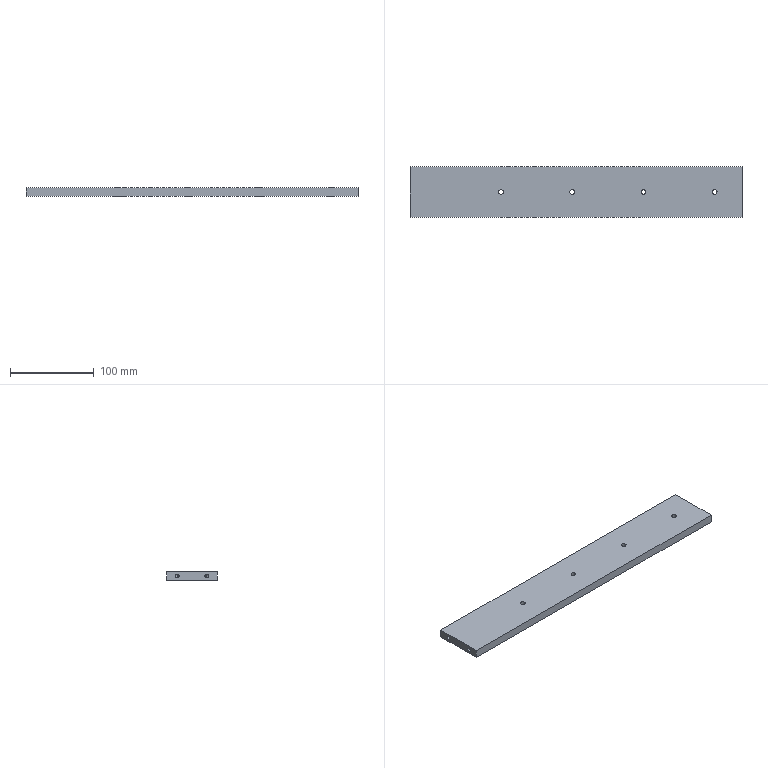Part | SolidWorks | features HoleWzd 2, Extrusion 1, MirrorPattern 1 | 1 solid | 42 faces | box 396 x 60 x 10 mm | volume 234690 mm3 | cylinder 24 | plane 10 | cone 8 | commonest cylinder face diameters 4.2 x8 5.5 x8 10 x8
STEP:
#1=CARTESIAN_POINT('',(185.6,17.5,7.1));
#2=VERTEX_POINT('',#1);
#3=CARTESIAN_POINT('',(185.6,17.5,2.9));
#4=VERTEX_POINT('',#3);
#5=CARTESIAN_POINT('',(185.6,17.5,5.));
#6=DIRECTION('',(1.,0.,0.));
#7=DIRECTION('',(0.,0.,-1.));
#8=AXIS2_PLACEMENT_3D('',#5,#6,#7);
#9=CIRCLE('',#8,2.1);
#10=EDGE_CURVE('',#2,#4,#9,.T.);
#11=ORIENTED_EDGE('',*,*,#10,.F.);
#12=CARTESIAN_POINT('',(198.,17.5,7.1));
#13=VERTEX_POINT('',#12);
#14=CARTESIAN_POINT('',(198.,17.5,7.1));
#15=DIRECTION('',(1.,0.,0.));
#16=VECTOR('',#15,1000.);
#17=LINE('',#14,#16);
#18=EDGE_CURVE('',#2,#13,#17,.T.);
#19=ORIENTED_EDGE('',*,*,#18,.T.);
#20=CARTESIAN_POINT('',(198.,17.5,2.9));
#21=VERTEX_POINT('',#20);
#22=CARTESIAN_POINT('',(198.,17.5,5.));
#23=DIRECTION('',(1.,0.,0.));
#24=DIRECTION('',(0.,0.,-1.));
#25=AXIS2_PLACEMENT_3D('',#22,#23,#24);
#26=CIRCLE('',#25,2.1);
#27=EDGE_CURVE('',#13,#21,#26,.T.);
#28=ORIENTED_EDGE('',*,*,#27,.T.);
#29=CARTESIAN_POINT('',(198.,17.5,2.9));
#30=DIRECTION('',(1.,0.,0.));
#31=VECTOR('',#30,1000.);
#32=LINE('',#29,#31);
#33=EDGE_CURVE('',#4,#21,#32,.T.);
#34=ORIENTED_EDGE('',*,*,#33,.F.);
#35=EDGE_LOOP('',(#11,#19,#28,#34));
#36=FACE_OUTER_BOUND('',#35,.T.);
#37=CARTESIAN_POINT('',(198.,17.5,5.));
#38=DIRECTION('',(1.,0.,0.));
#39=DIRECTION('',(0.,0.,-1.));
#40=AXIS2_PLACEMENT_3D('',#37,#38,#39);
#41=CYLINDRICAL_SURFACE('',#40,2.1);
#42=ADVANCED_FACE('',(#36),#41,.F.);
#43=CARTESIAN_POINT('',(184.338,17.5,5.));
#44=VERTEX_POINT('',#43);
#45=CARTESIAN_POINT('',(185.6,17.5,2.9));
#46=DIRECTION('',(0.515,0.,-0.8572));
#47=VECTOR('',#46,1000.);
#48=LINE('',#45,#47);
#49=EDGE_CURVE('',#44,#4,#48,.T.);
#50=ORIENTED_EDGE('',*,*,#49,.F.);
#51=CARTESIAN_POINT('',(185.6,17.5,7.1));
#52=DIRECTION('',(0.515,0.,0.8572));
#53=VECTOR('',#52,1000.);
#54=LINE('',#51,#53);
#55=EDGE_CURVE('',#44,#2,#54,.T.);
#56=ORIENTED_EDGE('',*,*,#55,.T.);
#57=ORIENTED_EDGE('',*,*,#10,.T.);
#58=EDGE_LOOP('',(#50,#56,#57));
#59=FACE_OUTER_BOUND('',#58,.T.);
#60=CARTESIAN_POINT('',(185.6,17.5,5.));
#61=DIRECTION('',(1.,0.,0.));
#62=DIRECTION('',(0.,0.,-1.));
#63=AXIS2_PLACEMENT_3D('',#60,#61,#62);
#64=CONICAL_SURFACE('',#63,2.1,1.03);
#65=ADVANCED_FACE('',(#59),#64,.F.);
#66=CARTESIAN_POINT('',(185.6,-17.5,7.1));
#67=VERTEX_POINT('',#66);
#68=CARTESIAN_POINT('',(185.6,-17.5,2.9));
#69=VERTEX_POINT('',#68);
#70=CARTESIAN_POINT('',(185.6,-17.5,5.));
#71=DIRECTION('',(1.,0.,0.));
#72=DIRECTION('',(0.,0.,-1.));
#73=AXIS2_PLACEMENT_3D('',#70,#71,#72);
#74=CIRCLE('',#73,2.1);
#75=EDGE_CURVE('',#67,#69,#74,.T.);
#76=ORIENTED_EDGE('',*,*,#75,.F.);
#77=CARTESIAN_POINT('',(198.,-17.5,7.1));
#78=VERTEX_POINT('',#77);
#79=CARTESIAN_POINT('',(198.,-17.5,7.1));
#80=DIRECTION('',(1.,0.,0.));
#81=VECTOR('',#80,1000.);
#82=LINE('',#79,#81);
#83=EDGE_CURVE('',#67,#78,#82,.T.);
#84=ORIENTED_EDGE('',*,*,#83,.T.);
#85=CARTESIAN_POINT('',(198.,-17.5,2.9));
#86=VERTEX_POINT('',#85);
#87=CARTESIAN_POINT('',(198.,-17.5,5.));
#88=DIRECTION('',(1.,0.,0.));
#89=DIRECTION('',(0.,0.,-1.));
#90=AXIS2_PLACEMENT_3D('',#87,#88,#89);
#91=CIRCLE('',#90,2.1);
#92=EDGE_CURVE('',#78,#86,#91,.T.);
#93=ORIENTED_EDGE('',*,*,#92,.T.);
#94=CARTESIAN_POINT('',(198.,-17.5,2.9));
#95=DIRECTION('',(1.,0.,0.));
#96=VECTOR('',#95,1000.);
#97=LINE('',#94,#96);
#98=EDGE_CURVE('',#69,#86,#97,.T.);
#99=ORIENTED_EDGE('',*,*,#98,.F.);
#100=EDGE_LOOP('',(#76,#84,#93,#99));
#101=FACE_OUTER_BOUND('',#100,.T.);
#102=CARTESIAN_POINT('',(198.,-17.5,5.));
#103=DIRECTION('',(1.,0.,0.));
#104=DIRECTION('',(0.,0.,-1.));
#105=AXIS2_PLACEMENT_3D('',#102,#103,#104);
#106=CYLINDRICAL_SURFACE('',#105,2.1);
#107=ADVANCED_FACE('',(#101),#106,.F.);
#108=CARTESIAN_POINT('',(184.338,-17.5,5.));
#109=VERTEX_POINT('',#108);
#110=CARTESIAN_POINT('',(185.6,-17.5,2.9));
#111=DIRECTION('',(0.515,0.,-0.8572));
#112=VECTOR('',#111,1000.);
#113=LINE('',#110,#112);
#114=EDGE_CURVE('',#109,#69,#113,.T.);
#115=ORIENTED_EDGE('',*,*,#114,.F.);
#116=CARTESIAN_POINT('',(185.6,-17.5,7.1));
#117=DIRECTION('',(0.515,0.,0.8572));
#118=VECTOR('',#117,1000.);
#119=LINE('',#116,#118);
#120=EDGE_CURVE('',#109,#67,#119,.T.);
#121=ORIENTED_EDGE('',*,*,#120,.T.);
#122=ORIENTED_EDGE('',*,*,#75,.T.);
#123=EDGE_LOOP('',(#115,#121,#122));
#124=FACE_OUTER_BOUND('',#123,.T.);
#125=CARTESIAN_POINT('',(185.6,-17.5,5.));
#126=DIRECTION('',(1.,0.,0.));
#127=DIRECTION('',(0.,0.,-1.));
#128=AXIS2_PLACEMENT_3D('',#125,#126,#127);
#129=CONICAL_SURFACE('',#128,2.1,1.03);
#130=ADVANCED_FACE('',(#124),#129,.F.);
#131=CARTESIAN_POINT('',(-185.6,17.5,2.9));
#132=VERTEX_POINT('',#131);
#133=CARTESIAN_POINT('',(-185.6,17.5,7.1));
#134=VERTEX_POINT('',#133);
#135=CARTESIAN_POINT('',(-185.6,17.5,5.));
#136=DIRECTION('',(-1.,0.,0.));
#137=DIRECTION('',(0.,0.,1.));
#138=AXIS2_PLACEMENT_3D('',#135,#136,#137);
#139=CIRCLE('',#138,2.1);
#140=EDGE_CURVE('',#132,#134,#139,.T.);
#141=ORIENTED_EDGE('',*,*,#140,.F.);
#142=CARTESIAN_POINT('',(-198.,17.5,2.9));
#143=VERTEX_POINT('',#142);
#144=CARTESIAN_POINT('',(-198.,17.5,2.9));
#145=DIRECTION('',(-1.,0.,0.));
#146=VECTOR('',#145,1000.);
#147=LINE('',#144,#146);
#148=EDGE_CURVE('',#132,#143,#147,.T.);
#149=ORIENTED_EDGE('',*,*,#148,.T.);
#150=CARTESIAN_POINT('',(-198.,17.5,7.1));
#151=VERTEX_POINT('',#150);
#152=CARTESIAN_POINT('',(-198.,17.5,5.));
#153=DIRECTION('',(-1.,0.,0.));
#154=DIRECTION('',(0.,0.,1.));
#155=AXIS2_PLACEMENT_3D('',#152,#153,#154);
#156=CIRCLE('',#155,2.1);
#157=EDGE_CURVE('',#143,#151,#156,.T.);
#158=ORIENTED_EDGE('',*,*,#157,.T.);
#159=CARTESIAN_POINT('',(-198.,17.5,7.1));
#160=DIRECTION('',(-1.,0.,0.));
#161=VECTOR('',#160,1000.);
#162=LINE('',#159,#161);
#163=EDGE_CURVE('',#134,#151,#162,.T.);
#164=ORIENTED_EDGE('',*,*,#163,.F.);
#165=EDGE_LOOP('',(#141,#149,#158,#164));
#166=FACE_OUTER_BOUND('',#165,.T.);
#167=CARTESIAN_POINT('',(-198.,17.5,5.));
#168=DIRECTION('',(-1.,0.,0.));
#169=DIRECTION('',(0.,0.,1.));
#170=AXIS2_PLACEMENT_3D('',#167,#168,#169);
#171=CYLINDRICAL_SURFACE('',#170,2.1);
#172=ADVANCED_FACE('',(#166),#171,.F.);
#173=CARTESIAN_POINT('',(-184.338,17.5,5.));
#174=VERTEX_POINT('',#173);
#175=CARTESIAN_POINT('',(-185.6,17.5,7.1));
#176=DIRECTION('',(-0.515,0.,0.8572));
#177=VECTOR('',#176,1000.);
#178=LINE('',#175,#177);
#179=EDGE_CURVE('',#174,#134,#178,.T.);
#180=ORIENTED_EDGE('',*,*,#179,.F.);
#181=CARTESIAN_POINT('',(-185.6,17.5,2.9));
#182=DIRECTION('',(-0.515,0.,-0.8572));
#183=VECTOR('',#182,1000.);
#184=LINE('',#181,#183);
#185=EDGE_CURVE('',#174,#132,#184,.T.);
#186=ORIENTED_EDGE('',*,*,#185,.T.);
#187=ORIENTED_EDGE('',*,*,#140,.T.);
#188=EDGE_LOOP('',(#180,#186,#187));
#189=FACE_OUTER_BOUND('',#188,.T.);
#190=CARTESIAN_POINT('',(-185.6,17.5,5.));
#191=DIRECTION('',(-1.,0.,0.));
#192=DIRECTION('',(0.,0.,1.));
#193=AXIS2_PLACEMENT_3D('',#190,#191,#192);
#194=CONICAL_SURFACE('',#193,2.1,1.03);
#195=ADVANCED_FACE('',(#189),#194,.F.);
#196=CARTESIAN_POINT('',(-185.6,-17.5,2.9));
#197=VERTEX_POINT('',#196);
#198=CARTESIAN_POINT('',(-185.6,-17.5,7.1));
#199=VERTEX_POINT('',#198);
#200=CARTESIAN_POINT('',(-185.6,-17.5,5.));
#201=DIRECTION('',(-1.,0.,0.));
#202=DIRECTION('',(0.,0.,1.));
#203=AXIS2_PLACEMENT_3D('',#200,#201,#202);
#204=CIRCLE('',#203,2.1);
#205=EDGE_CURVE('',#197,#199,#204,.T.);
#206=ORIENTED_EDGE('',*,*,#205,.F.);
#207=CARTESIAN_POINT('',(-198.,-17.5,2.9));
#208=VERTEX_POINT('',#207);
#209=CARTESIAN_POINT('',(-198.,-17.5,2.9));
#210=DIRECTION('',(-1.,0.,0.));
#211=VECTOR('',#210,1000.);
#212=LINE('',#209,#211);
#213=EDGE_CURVE('',#197,#208,#212,.T.);
#214=ORIENTED_EDGE('',*,*,#213,.T.);
#215=CARTESIAN_POINT('',(-198.,-17.5,7.1));
#216=VERTEX_POINT('',#215);
#217=CARTESIAN_POINT('',(-198.,-17.5,5.));
#218=DIRECTION('',(-1.,0.,0.));
#219=DIRECTION('',(0.,0.,1.));
#220=AXIS2_PLACEMENT_3D('',#217,#218,#219);
#221=CIRCLE('',#220,2.1);
#222=EDGE_CURVE('',#208,#216,#221,.T.);
#223=ORIENTED_EDGE('',*,*,#222,.T.);
#224=CARTESIAN_POINT('',(-198.,-17.5,7.1));
#225=DIRECTION('',(-1.,0.,0.));
#226=VECTOR('',#225,1000.);
#227=LINE('',#224,#226);
#228=EDGE_CURVE('',#199,#216,#227,.T.);
#229=ORIENTED_EDGE('',*,*,#228,.F.);
#230=EDGE_LOOP('',(#206,#214,#223,#229));
#231=FACE_OUTER_BOUND('',#230,.T.);
#232=CARTESIAN_POINT('',(-198.,-17.5,5.));
#233=DIRECTION('',(-1.,0.,0.));
#234=DIRECTION('',(0.,0.,1.));
#235=AXIS2_PLACEMENT_3D('',#232,#233,#234);
#236=CYLINDRICAL_SURFACE('',#235,2.1);
#237=ADVANCED_FACE('',(#231),#236,.F.);
#238=CARTESIAN_POINT('',(-184.338,-17.5,5.));
#239=VERTEX_POINT('',#238);
#240=CARTESIAN_POINT('',(-185.6,-17.5,7.1));
#241=DIRECTION('',(-0.515,0.,0.8572));
#242=VECTOR('',#241,1000.);
#243=LINE('',#240,#242);
#244=EDGE_CURVE('',#239,#199,#243,.T.);
#245=ORIENTED_EDGE('',*,*,#244,.F.);
#246=CARTESIAN_POINT('',(-185.6,-17.5,2.9));
#247=DIRECTION('',(-0.515,0.,-0.8572));
#248=VECTOR('',#247,1000.);
#249=LINE('',#246,#248);
#250=EDGE_CURVE('',#239,#197,#249,.T.);
#251=ORIENTED_EDGE('',*,*,#250,.T.);
#252=ORIENTED_EDGE('',*,*,#205,.T.);
#253=EDGE_LOOP('',(#245,#251,#252));
#254=FACE_OUTER_BOUND('',#253,.T.);
#255=CARTESIAN_POINT('',(-185.6,-17.5,5.));
#256=DIRECTION('',(-1.,0.,0.));
#257=DIRECTION('',(0.,0.,1.));
#258=AXIS2_PLACEMENT_3D('',#255,#256,#257);
#259=CONICAL_SURFACE('',#258,2.1,1.03);
#260=ADVANCED_FACE('',(#254),#259,.F.);
#261=CARTESIAN_POINT('',(-84.5,0.,5.7));
#262=VERTEX_POINT('',#261);
#263=CARTESIAN_POINT('',(-94.5,0.,5.7));
#264=VERTEX_POINT('',#263);
#265=CARTESIAN_POINT('',(-89.5,0.,5.7));
#266=DIRECTION('',(0.,0.,-1.));
#267=DIRECTION('',(-1.,0.,0.));
#268=AXIS2_PLACEMENT_3D('',#265,#266,#267);
#269=CIRCLE('',#268,5.);
#270=EDGE_CURVE('',#262,#264,#269,.T.);
#271=ORIENTED_EDGE('',*,*,#270,.F.);
#272=CARTESIAN_POINT('',(-84.5,0.,0.));
#273=VERTEX_POINT('',#272);
#274=CARTESIAN_POINT('',(-84.5,0.,0.));
#275=DIRECTION('',(0.,0.,-1.));
#276=VECTOR('',#275,1000.);
#277=LINE('',#274,#276);
#278=EDGE_CURVE('',#262,#273,#277,.T.);
#279=ORIENTED_EDGE('',*,*,#278,.T.);
#280=CARTESIAN_POINT('',(-94.5,0.,0.));
#281=VERTEX_POINT('',#280);
#282=CARTESIAN_POINT('',(-89.5,0.,0.));
#283=DIRECTION('',(0.,0.,-1.));
#284=DIRECTION('',(-1.,0.,0.));
#285=AXIS2_PLACEMENT_3D('',#282,#283,#284);
#286=CIRCLE('',#285,5.);
#287=EDGE_CURVE('',#273,#281,#286,.T.);
#288=ORIENTED_EDGE('',*,*,#287,.T.);
#289=CARTESIAN_POINT('',(-94.5,0.,0.));
#290=DIRECTION('',(0.,0.,-1.));
#291=VECTOR('',#290,1000.);
#292=LINE('',#289,#291);
#293=EDGE_CURVE('',#264,#281,#292,.T.);
#294=ORIENTED_EDGE('',*,*,#293,.F.);
#295=EDGE_LOOP('',(#271,#279,#288,#294));
#296=FACE_OUTER_BOUND('',#295,.T.);
#297=CARTESIAN_POINT('',(-89.5,0.,0.));
#298=DIRECTION('',(0.,0.,-1.));
#299=DIRECTION('',(-1.,0.,0.));
#300=AXIS2_PLACEMENT_3D('',#297,#298,#299);
#301=CYLINDRICAL_SURFACE('',#300,5.);
#302=ADVANCED_FACE('',(#296),#301,.F.);
#303=CARTESIAN_POINT('',(-86.75,0.,10.));
#304=VERTEX_POINT('',#303);
#305=CARTESIAN_POINT('',(-92.25,0.,10.));
#306=VERTEX_POINT('',#305);
#307=CARTESIAN_POINT('',(-89.5,0.,10.));
#308=DIRECTION('',(0.,0.,-1.));
#309=DIRECTION('',(-1.,0.,0.));
#310=AXIS2_PLACEMENT_3D('',#307,#308,#309);
#311=CIRCLE('',#310,2.75);
#312=EDGE_CURVE('',#304,#306,#311,.T.);
#313=ORIENTED_EDGE('',*,*,#312,.F.);
#314=CARTESIAN_POINT('',(-86.75,0.,5.7));
#315=VERTEX_POINT('',#314);
#316=CARTESIAN_POINT('',(-86.75,0.,0.));
#317=DIRECTION('',(0.,0.,-1.));
#318=VECTOR('',#317,1000.);
#319=LINE('',#316,#318);
#320=EDGE_CURVE('',#304,#315,#319,.T.);
#321=ORIENTED_EDGE('',*,*,#320,.T.);
#322=CARTESIAN_POINT('',(-92.25,0.,5.7));
#323=VERTEX_POINT('',#322);
#324=CARTESIAN_POINT('',(-89.5,0.,5.7));
#325=DIRECTION('',(0.,0.,-1.));
#326=DIRECTION('',(-1.,0.,0.));
#327=AXIS2_PLACEMENT_3D('',#324,#325,#326);
#328=CIRCLE('',#327,2.75);
#329=EDGE_CURVE('',#315,#323,#328,.T.);
#330=ORIENTED_EDGE('',*,*,#329,.T.);
#331=CARTESIAN_POINT('',(-92.25,0.,0.));
#332=DIRECTION('',(0.,0.,-1.));
#333=VECTOR('',#332,1000.);
#334=LINE('',#331,#333);
#335=EDGE_CURVE('',#306,#323,#334,.T.);
#336=ORIENTED_EDGE('',*,*,#335,.F.);
#337=EDGE_LOOP('',(#313,#321,#330,#336));
#338=FACE_OUTER_BOUND('',#337,.T.);
#339=CARTESIAN_POINT('',(-89.5,0.,0.));
#340=DIRECTION('',(0.,0.,-1.));
#341=DIRECTION('',(-1.,0.,0.));
#342=AXIS2_PLACEMENT_3D('',#339,#340,#341);
#343=CYLINDRICAL_SURFACE('',#342,2.75);
#344=ADVANCED_FACE('',(#338),#343,.F.);
#345=CARTESIAN_POINT('',(0.5,0.,5.7));
#346=VERTEX_POINT('',#345);
#347=CARTESIAN_POINT('',(-9.5,0.,5.7));
#348=VERTEX_POINT('',#347);
#349=CARTESIAN_POINT('',(-4.5,0.,5.7));
#350=DIRECTION('',(0.,0.,-1.));
#351=DIRECTION('',(-1.,0.,0.));
#352=AXIS2_PLACEMENT_3D('',#349,#350,#351);
#353=CIRCLE('',#352,5.);
#354=EDGE_CURVE('',#346,#348,#353,.T.);
#355=ORIENTED_EDGE('',*,*,#354,.F.);
#356=CARTESIAN_POINT('',(0.5,0.,0.));
#357=VERTEX_POINT('',#356);
#358=CARTESIAN_POINT('',(0.5,0.,0.));
#359=DIRECTION('',(0.,0.,-1.));
#360=VECTOR('',#359,1000.);
#361=LINE('',#358,#360);
#362=EDGE_CURVE('',#346,#357,#361,.T.);
#363=ORIENTED_EDGE('',*,*,#362,.T.);
#364=CARTESIAN_POINT('',(-9.5,0.,0.));
#365=VERTEX_POINT('',#364);
#366=CARTESIAN_POINT('',(-4.5,0.,0.));
#367=DIRECTION('',(0.,0.,-1.));
#368=DIRECTION('',(-1.,0.,0.));
#369=AXIS2_PLACEMENT_3D('',#366,#367,#368);
#370=CIRCLE('',#369,5.);
#371=EDGE_CURVE('',#357,#365,#370,.T.);
#372=ORIENTED_EDGE('',*,*,#371,.T.);
#373=CARTESIAN_POINT('',(-9.5,0.,0.));
#374=DIRECTION('',(0.,0.,-1.));
#375=VECTOR('',#374,1000.);
#376=LINE('',#373,#375);
#377=EDGE_CURVE('',#348,#365,#376,.T.);
#378=ORIENTED_EDGE('',*,*,#377,.F.);
#379=EDGE_LOOP('',(#355,#363,#372,#378));
#380=FACE_OUTER_BOUND('',#379,.T.);
#381=CARTESIAN_POINT('',(-4.5,0.,0.));
#382=DIRECTION('',(0.,0.,-1.));
#383=DIRECTION('',(-1.,0.,0.));
#384=AXIS2_PLACEMENT_3D('',#381,#382,#383);
#385=CYLINDRICAL_SURFACE('',#384,5.);
#386=ADVANCED_FACE('',(#380),#385,.F.);
#387=CARTESIAN_POINT('',(-1.75,0.,10.));
#388=VERTEX_POINT('',#387);
#389=CARTESIAN_POINT('',(-7.25,0.,10.));
#390=VERTEX_POINT('',#389);
#391=CARTESIAN_POINT('',(-4.5,0.,10.));
#392=DIRECTION('',(0.,0.,-1.));
#393=DIRECTION('',(-1.,0.,0.));
#394=AXIS2_PLACEMENT_3D('',#391,#392,#393);
#395=CIRCLE('',#394,2.75);
#396=EDGE_CURVE('',#388,#390,#395,.T.);
#397=ORIENTED_EDGE('',*,*,#396,.F.);
#398=CARTESIAN_POINT('',(-1.75,0.,5.7));
#399=VERTEX_POINT('',#398);
#400=CARTESIAN_POINT('',(-1.75,0.,0.));
#401=DIRECTION('',(0.,0.,-1.));
#402=VECTOR('',#401,1000.);
#403=LINE('',#400,#402);
#404=EDGE_CURVE('',#388,#399,#403,.T.);
#405=ORIENTED_EDGE('',*,*,#404,.T.);
#406=CARTESIAN_POINT('',(-7.25,0.,5.7));
#407=VERTEX_POINT('',#406);
#408=CARTESIAN_POINT('',(-4.5,0.,5.7));
#409=DIRECTION('',(0.,0.,-1.));
#410=DIRECTION('',(-1.,0.,0.));
#411=AXIS2_PLACEMENT_3D('',#408,#409,#410);
#412=CIRCLE('',#411,2.75);
#413=EDGE_CURVE('',#399,#407,#412,.T.);
#414=ORIENTED_EDGE('',*,*,#413,.T.);
#415=CARTESIAN_POINT('',(-7.25,0.,0.));
#416=DIRECTION('',(0.,0.,-1.));
#417=VECTOR('',#416,1000.);
#418=LINE('',#415,#417);
#419=EDGE_CURVE('',#390,#407,#418,.T.);
#420=ORIENTED_EDGE('',*,*,#419,.F.);
#421=EDGE_LOOP('',(#397,#405,#414,#420));
#422=FACE_OUTER_BOUND('',#421,.T.);
#423=CARTESIAN_POINT('',(-4.5,0.,0.));
#424=DIRECTION('',(0.,0.,-1.));
#425=DIRECTION('',(-1.,0.,0.));
#426=AXIS2_PLACEMENT_3D('',#423,#424,#425);
#427=CYLINDRICAL_SURFACE('',#426,2.75);
#428=ADVANCED_FACE('',(#422),#427,.F.);
#429=CARTESIAN_POINT('',(85.5,0.,5.7));
#430=VERTEX_POINT('',#429);
#431=CARTESIAN_POINT('',(75.5,0.,5.7));
#432=VERTEX_POINT('',#431);
#433=CARTESIAN_POINT('',(80.5,0.,5.7));
#434=DIRECTION('',(0.,0.,-1.));
#435=DIRECTION('',(-1.,0.,0.));
#436=AXIS2_PLACEMENT_3D('',#433,#434,#435);
#437=CIRCLE('',#436,5.);
#438=EDGE_CURVE('',#430,#432,#437,.T.);
#439=ORIENTED_EDGE('',*,*,#438,.F.);
#440=CARTESIAN_POINT('',(85.5,0.,0.));
#441=VERTEX_POINT('',#440);
#442=CARTESIAN_POINT('',(85.5,0.,0.));
#443=DIRECTION('',(0.,0.,-1.));
#444=VECTOR('',#443,1000.);
#445=LINE('',#442,#444);
#446=EDGE_CURVE('',#430,#441,#445,.T.);
#447=ORIENTED_EDGE('',*,*,#446,.T.);
#448=CARTESIAN_POINT('',(75.5,0.,0.));
#449=VERTEX_POINT('',#448);
#450=CARTESIAN_POINT('',(80.5,0.,0.));
#451=DIRECTION('',(0.,0.,-1.));
#452=DIRECTION('',(-1.,0.,0.));
#453=AXIS2_PLACEMENT_3D('',#450,#451,#452);
#454=CIRCLE('',#453,5.);
#455=EDGE_CURVE('',#441,#449,#454,.T.);
#456=ORIENTED_EDGE('',*,*,#455,.T.);
#457=CARTESIAN_POINT('',(75.5,0.,0.));
#458=DIRECTION('',(0.,0.,-1.));
#459=VECTOR('',#458,1000.);
#460=LINE('',#457,#459);
#461=EDGE_CURVE('',#432,#449,#460,.T.);
#462=ORIENTED_EDGE('',*,*,#461,.F.);
#463=EDGE_LOOP('',(#439,#447,#456,#462));
#464=FACE_OUTER_BOUND('',#463,.T.);
#465=CARTESIAN_POINT('',(80.5,0.,0.));
#466=DIRECTION('',(0.,0.,-1.));
#467=DIRECTION('',(-1.,0.,0.));
#468=AXIS2_PLACEMENT_3D('',#465,#466,#467);
#469=CYLINDRICAL_SURFACE('',#468,5.);
#470=ADVANCED_FACE('',(#464),#469,.F.);
#471=CARTESIAN_POINT('',(83.25,0.,10.));
#472=VERTEX_POINT('',#471);
#473=CARTESIAN_POINT('',(77.75,0.,10.));
#474=VERTEX_POINT('',#473);
#475=CARTESIAN_POINT('',(80.5,0.,10.));
#476=DIRECTION('',(0.,0.,-1.));
#477=DIRECTION('',(-1.,0.,0.));
#478=AXIS2_PLACEMENT_3D('',#475,#476,#477);
#479=CIRCLE('',#478,2.75);
#480=EDGE_CURVE('',#472,#474,#479,.T.);
#481=ORIENTED_EDGE('',*,*,#480,.F.);
#482=CARTESIAN_POINT('',(83.25,0.,5.7));
#483=VERTEX_POINT('',#482);
#484=CARTESIAN_POINT('',(83.25,0.,0.));
#485=DIRECTION('',(0.,0.,-1.));
#486=VECTOR('',#485,1000.);
#487=LINE('',#484,#486);
#488=EDGE_CURVE('',#472,#483,#487,.T.);
#489=ORIENTED_EDGE('',*,*,#488,.T.);
#490=CARTESIAN_POINT('',(77.75,0.,5.7));
#491=VERTEX_POINT('',#490);
#492=CARTESIAN_POINT('',(80.5,0.,5.7));
#493=DIRECTION('',(0.,0.,-1.));
#494=DIRECTION('',(-1.,0.,0.));
#495=AXIS2_PLACEMENT_3D('',#492,#493,#494);
#496=CIRCLE('',#495,2.75);
#497=EDGE_CURVE('',#483,#491,#496,.T.);
#498=ORIENTED_EDGE('',*,*,#497,.T.);
#499=CARTESIAN_POINT('',(77.75,0.,0.));
#500=DIRECTION('',(0.,0.,-1.));
#501=VECTOR('',#500,1000.);
#502=LINE('',#499,#501);
#503=EDGE_CURVE('',#474,#491,#502,.T.);
#504=ORIENTED_EDGE('',*,*,#503,.F.);
#505=EDGE_LOOP('',(#481,#489,#498,#504));
#506=FACE_OUTER_BOUND('',#505,.T.);
#507=CARTESIAN_POINT('',(80.5,0.,0.));
#508=DIRECTION('',(0.,0.,-1.));
#509=DIRECTION('',(-1.,0.,0.));
#510=AXIS2_PLACEMENT_3D('',#507,#508,#509);
#511=CYLINDRICAL_SURFACE('',#510,2.75);
#512=ADVANCED_FACE('',(#506),#511,.F.);
#513=CARTESIAN_POINT('',(170.5,0.,5.7));
#514=VERTEX_POINT('',#513);
#515=CARTESIAN_POINT('',(160.5,0.,5.7));
#516=VERTEX_POINT('',#515);
#517=CARTESIAN_POINT('',(165.5,0.,5.7));
#518=DIRECTION('',(0.,0.,-1.));
#519=DIRECTION('',(-1.,0.,0.));
#520=AXIS2_PLACEMENT_3D('',#517,#518,#519);
#521=CIRCLE('',#520,5.);
#522=EDGE_CURVE('',#514,#516,#521,.T.);
#523=ORIENTED_EDGE('',*,*,#522,.F.);
#524=CARTESIAN_POINT('',(170.5,0.,0.));
#525=VERTEX_POINT('',#524);
#526=CARTESIAN_POINT('',(170.5,0.,0.));
#527=DIRECTION('',(0.,0.,-1.));
#528=VECTOR('',#527,1000.);
#529=LINE('',#526,#528);
#530=EDGE_CURVE('',#514,#525,#529,.T.);
#531=ORIENTED_EDGE('',*,*,#530,.T.);
#532=CARTESIAN_POINT('',(160.5,0.,0.));
#533=VERTEX_POINT('',#532);
#534=CARTESIAN_POINT('',(165.5,0.,0.));
#535=DIRECTION('',(0.,0.,-1.));
#536=DIRECTION('',(-1.,0.,0.));
#537=AXIS2_PLACEMENT_3D('',#534,#535,#536);
#538=CIRCLE('',#537,5.);
#539=EDGE_CURVE('',#525,#533,#538,.T.);
#540=ORIENTED_EDGE('',*,*,#539,.T.);
#541=CARTESIAN_POINT('',(160.5,0.,0.));
#542=DIRECTION('',(0.,0.,-1.));
#543=VECTOR('',#542,1000.);
#544=LINE('',#541,#543);
#545=EDGE_CURVE('',#516,#533,#544,.T.);
#546=ORIENTED_EDGE('',*,*,#545,.F.);
#547=EDGE_LOOP('',(#523,#531,#540,#546));
#548=FACE_OUTER_BOUND('',#547,.T.);
#549=CARTESIAN_POINT('',(165.5,0.,0.));
#550=DIRECTION('',(0.,0.,-1.));
#551=DIRECTION('',(-1.,0.,0.));
#552=AXIS2_PLACEMENT_3D('',#549,#550,#551);
#553=CYLINDRICAL_SURFACE('',#552,5.);
#554=ADVANCED_FACE('',(#548),#553,.F.);
#555=CARTESIAN_POINT('',(168.25,0.,10.));
#556=VERTEX_POINT('',#555);
#557=CARTESIAN_POINT('',(162.75,0.,10.));
#558=VERTEX_POINT('',#557);
#559=CARTESIAN_POINT('',(165.5,0.,10.));
#560=DIRECTION('',(0.,0.,-1.));
#561=DIRECTION('',(-1.,0.,0.));
#562=AXIS2_PLACEMENT_3D('',#559,#560,#561);
#563=CIRCLE('',#562,2.75);
#564=EDGE_CURVE('',#556,#558,#563,.T.);
#565=ORIENTED_EDGE('',*,*,#564,.F.);
#566=CARTESIAN_POINT('',(168.25,0.,5.7));
#567=VERTEX_POINT('',#566);
#568=CARTESIAN_POINT('',(168.25,0.,0.));
#569=DIRECTION('',(0.,0.,-1.));
#570=VECTOR('',#569,1000.);
#571=LINE('',#568,#570);
#572=EDGE_CURVE('',#556,#567,#571,.T.);
#573=ORIENTED_EDGE('',*,*,#572,.T.);
#574=CARTESIAN_POINT('',(162.75,0.,5.7));
#575=VERTEX_POINT('',#574);
#576=CARTESIAN_POINT('',(165.5,0.,5.7));
#577=DIRECTION('',(0.,0.,-1.));
#578=DIRECTION('',(-1.,0.,0.));
#579=AXIS2_PLACEMENT_3D('',#576,#577,#578);
#580=CIRCLE('',#579,2.75);
#581=EDGE_CURVE('',#567,#575,#580,.T.);
#582=ORIENTED_EDGE('',*,*,#581,.T.);
#583=CARTESIAN_POINT('',(162.75,0.,0.));
#584=DIRECTION('',(0.,0.,-1.));
#585=VECTOR('',#584,1000.);
#586=LINE('',#583,#585);
#587=EDGE_CURVE('',#558,#575,#586,.T.);
#588=ORIENTED_EDGE('',*,*,#587,.F.);
#589=EDGE_LOOP('',(#565,#573,#582,#588));
#590=FACE_OUTER_BOUND('',#589,.T.);
#591=CARTESIAN_POINT('',(165.5,0.,0.));
#592=DIRECTION('',(0.,0.,-1.));
#593=DIRECTION('',(-1.,0.,0.));
#594=AXIS2_PLACEMENT_3D('',#591,#592,#593);
#595=CYLINDRICAL_SURFACE('',#594,2.75);
#596=ADVANCED_FACE('',(#590),#595,.F.);
#597=CARTESIAN_POINT('',(198.,17.5,5.));
#598=DIRECTION('',(1.,0.,0.));
#599=DIRECTION('',(0.,0.,-1.));
#600=AXIS2_PLACEMENT_3D('',#597,#598,#599);
#601=CIRCLE('',#600,2.1);
#602=EDGE_CURVE('',#21,#13,#601,.T.);
#603=ORIENTED_EDGE('',*,*,#602,.F.);
#604=ORIENTED_EDGE('',*,*,#27,.F.);
#605=EDGE_LOOP('',(#603,#604));
#606=FACE_BOUND('',#605,.T.);
#607=CARTESIAN_POINT('',(198.,-17.5,5.));
#608=DIRECTION('',(1.,0.,0.));
#609=DIRECTION('',(0.,0.,-1.));
#610=AXIS2_PLACEMENT_3D('',#607,#608,#609);
#611=CIRCLE('',#610,2.1);
#612=EDGE_CURVE('',#86,#78,#611,.T.);
#613=ORIENTED_EDGE('',*,*,#612,.F.);
#614=ORIENTED_EDGE('',*,*,#92,.F.);
#615=EDGE_LOOP('',(#613,#614));
#616=FACE_BOUND('',#615,.T.);
#617=CARTESIAN_POINT('',(198.,-30.,0.));
#618=VERTEX_POINT('',#617);
#619=CARTESIAN_POINT('',(198.,30.,0.));
#620=VERTEX_POINT('',#619);
#621=CARTESIAN_POINT('',(198.,30.,0.));
#622=DIRECTION('',(0.,1.,0.));
#623=VECTOR('',#622,1000.);
#624=LINE('',#621,#623);
#625=EDGE_CURVE('',#618,#620,#624,.T.);
#626=ORIENTED_EDGE('',*,*,#625,.T.);
#627=CARTESIAN_POINT('',(198.,30.,10.));
#628=VERTEX_POINT('',#627);
#629=CARTESIAN_POINT('',(198.,30.,10.));
#630=DIRECTION('',(0.,0.,-1.));
#631=VECTOR('',#630,1000.);
#632=LINE('',#629,#631);
#633=EDGE_CURVE('',#628,#620,#632,.T.);
#634=ORIENTED_EDGE('',*,*,#633,.F.);
#635=CARTESIAN_POINT('',(198.,-30.,10.));
#636=VERTEX_POINT('',#635);
#637=CARTESIAN_POINT('',(198.,30.,10.));
#638=DIRECTION('',(0.,1.,0.));
#639=VECTOR('',#638,1000.);
#640=LINE('',#637,#639);
#641=EDGE_CURVE('',#636,#628,#640,.T.);
#642=ORIENTED_EDGE('',*,*,#641,.F.);
#643=CARTESIAN_POINT('',(198.,-30.,10.));
#644=DIRECTION('',(0.,0.,-1.));
#645=VECTOR('',#644,1000.);
#646=LINE('',#643,#645);
#647=EDGE_CURVE('',#636,#618,#646,.T.);
#648=ORIENTED_EDGE('',*,*,#647,.T.);
#649=EDGE_LOOP('',(#626,#634,#642,#648));
#650=FACE_OUTER_BOUND('',#649,.T.);
#651=CARTESIAN_POINT('',(198.,30.,10.));
#652=DIRECTION('',(-1.,0.,0.));
#653=DIRECTION('',(0.,0.,1.));
#654=AXIS2_PLACEMENT_3D('',#651,#652,#653);
#655=PLANE('',#654);
#656=ADVANCED_FACE('',(#606,#616,#650),#655,.F.);
#657=CARTESIAN_POINT('',(-198.,30.,0.));
#658=VERTEX_POINT('',#657);
#659=CARTESIAN_POINT('',(-198.,30.,0.));
#660=DIRECTION('',(-1.,0.,0.));
#661=VECTOR('',#660,1000.);
#662=LINE('',#659,#661);
#663=EDGE_CURVE('',#620,#658,#662,.T.);
#664=ORIENTED_EDGE('',*,*,#663,.T.);
#665=CARTESIAN_POINT('',(-198.,30.,10.));
#666=VERTEX_POINT('',#665);
#667=CARTESIAN_POINT('',(-198.,30.,10.));
#668=DIRECTION('',(0.,0.,-1.));
#669=VECTOR('',#668,1000.);
#670=LINE('',#667,#669);
#671=EDGE_CURVE('',#666,#658,#670,.T.);
#672=ORIENTED_EDGE('',*,*,#671,.F.);
#673=CARTESIAN_POINT('',(-198.,30.,10.));
#674=DIRECTION('',(-1.,0.,0.));
#675=VECTOR('',#674,1000.);
#676=LINE('',#673,#675);
#677=EDGE_CURVE('',#628,#666,#676,.T.);
#678=ORIENTED_EDGE('',*,*,#677,.F.);
#679=ORIENTED_EDGE('',*,*,#633,.T.);
#680=EDGE_LOOP('',(#664,#672,#678,#679));
#681=FACE_OUTER_BOUND('',#680,.T.);
#682=CARTESIAN_POINT('',(-198.,30.,10.));
#683=DIRECTION('',(0.,-1.,0.));
#684=DIRECTION('',(0.,0.,-1.));
#685=AXIS2_PLACEMENT_3D('',#682,#683,#684);
#686=PLANE('',#685);
#687=ADVANCED_FACE('',(#681),#686,.F.);
#688=CARTESIAN_POINT('',(-198.,17.5,5.));
#689=DIRECTION('',(-1.,0.,0.));
#690=DIRECTION('',(0.,0.,1.));
#691=AXIS2_PLACEMENT_3D('',#688,#689,#690);
#692=CIRCLE('',#691,2.1);
#693=EDGE_CURVE('',#151,#143,#692,.T.);
#694=ORIENTED_EDGE('',*,*,#693,.F.);
#695=ORIENTED_EDGE('',*,*,#157,.F.);
#696=EDGE_LOOP('',(#694,#695));
#697=FACE_BOUND('',#696,.T.);
#698=CARTESIAN_POINT('',(-198.,-17.5,5.));
#699=DIRECTION('',(-1.,0.,0.));
#700=DIRECTION('',(0.,0.,1.));
#701=AXIS2_PLACEMENT_3D('',#698,#699,#700);
#702=CIRCLE('',#701,2.1);
#703=EDGE_CURVE('',#216,#208,#702,.T.);
#704=ORIENTED_EDGE('',*,*,#703,.F.);
#705=ORIENTED_EDGE('',*,*,#222,.F.);
#706=EDGE_LOOP('',(#704,#705));
#707=FACE_BOUND('',#706,.T.);
#708=CARTESIAN_POINT('',(-198.,-30.,0.));
#709=VERTEX_POINT('',#708);
#710=CARTESIAN_POINT('',(-198.,30.,0.));
#711=DIRECTION('',(0.,-1.,0.));
#712=VECTOR('',#711,1000.);
#713=LINE('',#710,#712);
#714=EDGE_CURVE('',#658,#709,#713,.T.);
#715=ORIENTED_EDGE('',*,*,#714,.T.);
#716=CARTESIAN_POINT('',(-198.,-30.,10.));
#717=VERTEX_POINT('',#716);
#718=CARTESIAN_POINT('',(-198.,-30.,10.));
#719=DIRECTION('',(0.,0.,-1.));
#720=VECTOR('',#719,1000.);
#721=LINE('',#718,#720);
#722=EDGE_CURVE('',#717,#709,#721,.T.);
#723=ORIENTED_EDGE('',*,*,#722,.F.);
#724=CARTESIAN_POINT('',(-198.,30.,10.));
#725=DIRECTION('',(0.,-1.,0.));
#726=VECTOR('',#725,1000.);
#727=LINE('',#724,#726);
#728=EDGE_CURVE('',#666,#717,#727,.T.);
#729=ORIENTED_EDGE('',*,*,#728,.F.);
#730=ORIENTED_EDGE('',*,*,#671,.T.);
#731=EDGE_LOOP('',(#715,#723,#729,#730));
#732=FACE_OUTER_BOUND('',#731,.T.);
#733=CARTESIAN_POINT('',(-198.,30.,10.));
#734=DIRECTION('',(1.,0.,0.));
#735=DIRECTION('',(0.,0.,-1.));
#736=AXIS2_PLACEMENT_3D('',#733,#734,#735);
#737=PLANE('',#736);
#738=ADVANCED_FACE('',(#697,#707,#732),#737,.F.);
#739=CARTESIAN_POINT('',(-198.,-30.,0.));
#740=DIRECTION('',(1.,0.,0.));
#741=VECTOR('',#740,1000.);
#742=LINE('',#739,#741);
#743=EDGE_CURVE('',#709,#618,#742,.T.);
#744=ORIENTED_EDGE('',*,*,#743,.T.);
#745=ORIENTED_EDGE('',*,*,#647,.F.);
#746=CARTESIAN_POINT('',(-198.,-30.,10.));
#747=DIRECTION('',(1.,0.,0.));
#748=VECTOR('',#747,1000.);
#749=LINE('',#746,#748);
#750=EDGE_CURVE('',#717,#636,#749,.T.);
#751=ORIENTED_EDGE('',*,*,#750,.F.);
#752=ORIENTED_EDGE('',*,*,#722,.T.);
#753=EDGE_LOOP('',(#744,#745,#751,#752));
#754=FACE_OUTER_BOUND('',#753,.T.);
#755=CARTESIAN_POINT('',(-198.,-30.,10.));
#756=DIRECTION('',(0.,1.,0.));
#757=DIRECTION('',(0.,0.,1.));
#758=AXIS2_PLACEMENT_3D('',#755,#756,#757);
#759=PLANE('',#758);
#760=ADVANCED_FACE('',(#754),#759,.F.);
#761=CARTESIAN_POINT('',(-89.5,0.,10.));
#762=DIRECTION('',(0.,0.,-1.));
#763=DIRECTION('',(-1.,0.,0.));
#764=AXIS2_PLACEMENT_3D('',#761,#762,#763);
#765=CIRCLE('',#764,2.75);
#766=EDGE_CURVE('',#306,#304,#765,.T.);
#767=ORIENTED_EDGE('',*,*,#766,.T.);
#768=ORIENTED_EDGE('',*,*,#312,.T.);
#769=EDGE_LOOP('',(#767,#768));
#770=FACE_BOUND('',#769,.T.);
#771=CARTESIAN_POINT('',(-4.5,0.,10.));
#772=DIRECTION('',(0.,0.,-1.));
#773=DIRECTION('',(-1.,0.,0.));
#774=AXIS2_PLACEMENT_3D('',#771,#772,#773);
#775=CIRCLE('',#774,2.75);
#776=EDGE_CURVE('',#390,#388,#775,.T.);
#777=ORIENTED_EDGE('',*,*,#776,.T.);
#778=ORIENTED_EDGE('',*,*,#396,.T.);
#779=EDGE_LOOP('',(#777,#778));
#780=FACE_BOUND('',#779,.T.);
#781=CARTESIAN_POINT('',(80.5,0.,10.));
#782=DIRECTION('',(0.,0.,-1.));
#783=DIRECTION('',(-1.,0.,0.));
#784=AXIS2_PLACEMENT_3D('',#781,#782,#783);
#785=CIRCLE('',#784,2.75);
#786=EDGE_CURVE('',#474,#472,#785,.T.);
#787=ORIENTED_EDGE('',*,*,#786,.T.);
#788=ORIENTED_EDGE('',*,*,#480,.T.);
#789=EDGE_LOOP('',(#787,#788));
#790=FACE_BOUND('',#789,.T.);
#791=CARTESIAN_POINT('',(165.5,0.,10.));
#792=DIRECTION('',(0.,0.,-1.));
#793=DIRECTION('',(-1.,0.,0.));
#794=AXIS2_PLACEMENT_3D('',#791,#792,#793);
#795=CIRCLE('',#794,2.75);
#796=EDGE_CURVE('',#558,#556,#795,.T.);
#797=ORIENTED_EDGE('',*,*,#796,.T.);
#798=ORIENTED_EDGE('',*,*,#564,.T.);
#799=EDGE_LOOP('',(#797,#798));
#800=FACE_BOUND('',#799,.T.);
#801=ORIENTED_EDGE('',*,*,#641,.T.);
#802=ORIENTED_EDGE('',*,*,#677,.T.);
#803=ORIENTED_EDGE('',*,*,#728,.T.);
#804=ORIENTED_EDGE('',*,*,#750,.T.);
#805=EDGE_LOOP('',(#801,#802,#803,#804));
#806=FACE_OUTER_BOUND('',#805,.T.);
#807=CARTESIAN_POINT('',(0.,0.,10.));
#808=DIRECTION('',(0.,0.,1.));
#809=DIRECTION('',(1.,0.,0.));
#810=AXIS2_PLACEMENT_3D('',#807,#808,#809);
#811=PLANE('',#810);
#812=ADVANCED_FACE('',(#770,#780,#790,#800,#806),#811,.T.);
#813=CARTESIAN_POINT('',(-89.5,0.,0.));
#814=DIRECTION('',(0.,0.,-1.));
#815=DIRECTION('',(-1.,0.,0.));
#816=AXIS2_PLACEMENT_3D('',#813,#814,#815);
#817=CIRCLE('',#816,5.);
#818=EDGE_CURVE('',#281,#273,#817,.T.);
#819=ORIENTED_EDGE('',*,*,#818,.F.);
#820=ORIENTED_EDGE('',*,*,#287,.F.);
#821=EDGE_LOOP('',(#819,#820));
#822=FACE_BOUND('',#821,.T.);
#823=CARTESIAN_POINT('',(-4.5,0.,0.));
#824=DIRECTION('',(0.,0.,-1.));
#825=DIRECTION('',(-1.,0.,0.));
#826=AXIS2_PLACEMENT_3D('',#823,#824,#825);
#827=CIRCLE('',#826,5.);
#828=EDGE_CURVE('',#365,#357,#827,.T.);
#829=ORIENTED_EDGE('',*,*,#828,.F.);
#830=ORIENTED_EDGE('',*,*,#371,.F.);
#831=EDGE_LOOP('',(#829,#830));
#832=FACE_BOUND('',#831,.T.);
#833=CARTESIAN_POINT('',(80.5,0.,0.));
#834=DIRECTION('',(0.,0.,-1.));
#835=DIRECTION('',(-1.,0.,0.));
#836=AXIS2_PLACEMENT_3D('',#833,#834,#835);
#837=CIRCLE('',#836,5.);
#838=EDGE_CURVE('',#449,#441,#837,.T.);
#839=ORIENTED_EDGE('',*,*,#838,.F.);
#840=ORIENTED_EDGE('',*,*,#455,.F.);
#841=EDGE_LOOP('',(#839,#840));
#842=FACE_BOUND('',#841,.T.);
#843=CARTESIAN_POINT('',(165.5,0.,0.));
#844=DIRECTION('',(0.,0.,-1.));
#845=DIRECTION('',(-1.,0.,0.));
#846=AXIS2_PLACEMENT_3D('',#843,#844,#845);
#847=CIRCLE('',#846,5.);
#848=EDGE_CURVE('',#533,#525,#847,.T.);
#849=ORIENTED_EDGE('',*,*,#848,.F.);
#850=ORIENTED_EDGE('',*,*,#539,.F.);
#851=EDGE_LOOP('',(#849,#850));
#852=FACE_BOUND('',#851,.T.);
#853=ORIENTED_EDGE('',*,*,#625,.F.);
#854=ORIENTED_EDGE('',*,*,#743,.F.);
#855=ORIENTED_EDGE('',*,*,#714,.F.);
#856=ORIENTED_EDGE('',*,*,#663,.F.);
#857=EDGE_LOOP('',(#853,#854,#855,#856));
#858=FACE_OUTER_BOUND('',#857,.T.);
#859=CARTESIAN_POINT('',(0.,0.,0.));
#860=DIRECTION('',(0.,0.,1.));
#861=DIRECTION('',(1.,0.,0.));
#862=AXIS2_PLACEMENT_3D('',#859,#860,#861);
#863=PLANE('',#862);
#864=ADVANCED_FACE('',(#822,#832,#842,#852,#858),#863,.F.);
#865=ORIENTED_EDGE('',*,*,#572,.F.);
#866=ORIENTED_EDGE('',*,*,#796,.F.);
#867=ORIENTED_EDGE('',*,*,#587,.T.);
#868=CARTESIAN_POINT('',(165.5,0.,5.7));
#869=DIRECTION('',(0.,0.,-1.));
#870=DIRECTION('',(-1.,0.,0.));
#871=AXIS2_PLACEMENT_3D('',#868,#869,#870);
#872=CIRCLE('',#871,2.75);
#873=EDGE_CURVE('',#575,#567,#872,.T.);
#874=ORIENTED_EDGE('',*,*,#873,.T.);
#875=EDGE_LOOP('',(#865,#866,#867,#874));
#876=FACE_OUTER_BOUND('',#875,.T.);
#877=CARTESIAN_POINT('',(165.5,0.,0.));
#878=DIRECTION('',(0.,0.,-1.));
#879=DIRECTION('',(-1.,0.,0.));
#880=AXIS2_PLACEMENT_3D('',#877,#878,#879);
#881=CYLINDRICAL_SURFACE('',#880,2.75);
#882=ADVANCED_FACE('',(#876),#881,.F.);
#883=ORIENTED_EDGE('',*,*,#873,.F.);
#884=ORIENTED_EDGE('',*,*,#581,.F.);
#885=EDGE_LOOP('',(#883,#884));
#886=FACE_BOUND('',#885,.T.);
#887=CARTESIAN_POINT('',(165.5,0.,5.7));
#888=DIRECTION('',(0.,0.,-1.));
#889=DIRECTION('',(-1.,0.,0.));
#890=AXIS2_PLACEMENT_3D('',#887,#888,#889);
#891=CIRCLE('',#890,5.);
#892=EDGE_CURVE('',#516,#514,#891,.T.);
#893=ORIENTED_EDGE('',*,*,#892,.T.);
#894=ORIENTED_EDGE('',*,*,#522,.T.);
#895=EDGE_LOOP('',(#893,#894));
#896=FACE_OUTER_BOUND('',#895,.T.);
#897=CARTESIAN_POINT('',(168.25,0.,5.7));
#898=DIRECTION('',(0.,0.,1.));
#899=DIRECTION('',(1.,0.,0.));
#900=AXIS2_PLACEMENT_3D('',#897,#898,#899);
#901=PLANE('',#900);
#902=ADVANCED_FACE('',(#886,#896),#901,.F.);
#903=ORIENTED_EDGE('',*,*,#530,.F.);
#904=ORIENTED_EDGE('',*,*,#892,.F.);
#905=ORIENTED_EDGE('',*,*,#545,.T.);
#906=ORIENTED_EDGE('',*,*,#848,.T.);
#907=EDGE_LOOP('',(#903,#904,#905,#906));
#908=FACE_OUTER_BOUND('',#907,.T.);
#909=CARTESIAN_POINT('',(165.5,0.,0.));
#910=DIRECTION('',(0.,0.,-1.));
#911=DIRECTION('',(-1.,0.,0.));
#912=AXIS2_PLACEMENT_3D('',#909,#910,#911);
#913=CYLINDRICAL_SURFACE('',#912,5.);
#914=ADVANCED_FACE('',(#908),#913,.F.);
#915=ORIENTED_EDGE('',*,*,#488,.F.);
#916=ORIENTED_EDGE('',*,*,#786,.F.);
#917=ORIENTED_EDGE('',*,*,#503,.T.);
#918=CARTESIAN_POINT('',(80.5,0.,5.7));
#919=DIRECTION('',(0.,0.,-1.));
#920=DIRECTION('',(-1.,0.,0.));
#921=AXIS2_PLACEMENT_3D('',#918,#919,#920);
#922=CIRCLE('',#921,2.75);
#923=EDGE_CURVE('',#491,#483,#922,.T.);
#924=ORIENTED_EDGE('',*,*,#923,.T.);
#925=EDGE_LOOP('',(#915,#916,#917,#924));
#926=FACE_OUTER_BOUND('',#925,.T.);
#927=CARTESIAN_POINT('',(80.5,0.,0.));
#928=DIRECTION('',(0.,0.,-1.));
#929=DIRECTION('',(-1.,0.,0.));
#930=AXIS2_PLACEMENT_3D('',#927,#928,#929);
#931=CYLINDRICAL_SURFACE('',#930,2.75);
#932=ADVANCED_FACE('',(#926),#931,.F.);
#933=ORIENTED_EDGE('',*,*,#923,.F.);
#934=ORIENTED_EDGE('',*,*,#497,.F.);
#935=EDGE_LOOP('',(#933,#934));
#936=FACE_BOUND('',#935,.T.);
#937=CARTESIAN_POINT('',(80.5,0.,5.7));
#938=DIRECTION('',(0.,0.,-1.));
#939=DIRECTION('',(-1.,0.,0.));
#940=AXIS2_PLACEMENT_3D('',#937,#938,#939);
#941=CIRCLE('',#940,5.);
#942=EDGE_CURVE('',#432,#430,#941,.T.);
#943=ORIENTED_EDGE('',*,*,#942,.T.);
#944=ORIENTED_EDGE('',*,*,#438,.T.);
#945=EDGE_LOOP('',(#943,#944));
#946=FACE_OUTER_BOUND('',#945,.T.);
#947=CARTESIAN_POINT('',(83.25,0.,5.7));
#948=DIRECTION('',(0.,0.,1.));
#949=DIRECTION('',(1.,0.,0.));
#950=AXIS2_PLACEMENT_3D('',#947,#948,#949);
#951=PLANE('',#950);
#952=ADVANCED_FACE('',(#936,#946),#951,.F.);
#953=ORIENTED_EDGE('',*,*,#446,.F.);
#954=ORIENTED_EDGE('',*,*,#942,.F.);
#955=ORIENTED_EDGE('',*,*,#461,.T.);
#956=ORIENTED_EDGE('',*,*,#838,.T.);
#957=EDGE_LOOP('',(#953,#954,#955,#956));
#958=FACE_OUTER_BOUND('',#957,.T.);
#959=CARTESIAN_POINT('',(80.5,0.,0.));
#960=DIRECTION('',(0.,0.,-1.));
#961=DIRECTION('',(-1.,0.,0.));
#962=AXIS2_PLACEMENT_3D('',#959,#960,#961);
#963=CYLINDRICAL_SURFACE('',#962,5.);
#964=ADVANCED_FACE('',(#958),#963,.F.);
#965=ORIENTED_EDGE('',*,*,#404,.F.);
#966=ORIENTED_EDGE('',*,*,#776,.F.);
#967=ORIENTED_EDGE('',*,*,#419,.T.);
#968=CARTESIAN_POINT('',(-4.5,0.,5.7));
#969=DIRECTION('',(0.,0.,-1.));
#970=DIRECTION('',(-1.,0.,0.));
#971=AXIS2_PLACEMENT_3D('',#968,#969,#970);
#972=CIRCLE('',#971,2.75);
#973=EDGE_CURVE('',#407,#399,#972,.T.);
#974=ORIENTED_EDGE('',*,*,#973,.T.);
#975=EDGE_LOOP('',(#965,#966,#967,#974));
#976=FACE_OUTER_BOUND('',#975,.T.);
#977=CARTESIAN_POINT('',(-4.5,0.,0.));
#978=DIRECTION('',(0.,0.,-1.));
#979=DIRECTION('',(-1.,0.,0.));
#980=AXIS2_PLACEMENT_3D('',#977,#978,#979);
#981=CYLINDRICAL_SURFACE('',#980,2.75);
#982=ADVANCED_FACE('',(#976),#981,.F.);
#983=ORIENTED_EDGE('',*,*,#973,.F.);
#984=ORIENTED_EDGE('',*,*,#413,.F.);
#985=EDGE_LOOP('',(#983,#984));
#986=FACE_BOUND('',#985,.T.);
#987=CARTESIAN_POINT('',(-4.5,0.,5.7));
#988=DIRECTION('',(0.,0.,-1.));
#989=DIRECTION('',(-1.,0.,0.));
#990=AXIS2_PLACEMENT_3D('',#987,#988,#989);
#991=CIRCLE('',#990,5.);
#992=EDGE_CURVE('',#348,#346,#991,.T.);
#993=ORIENTED_EDGE('',*,*,#992,.T.);
#994=ORIENTED_EDGE('',*,*,#354,.T.);
#995=EDGE_LOOP('',(#993,#994));
#996=FACE_OUTER_BOUND('',#995,.T.);
#997=CARTESIAN_POINT('',(-1.75,0.,5.7));
#998=DIRECTION('',(0.,0.,1.));
#999=DIRECTION('',(1.,0.,0.));
#1000=AXIS2_PLACEMENT_3D('',#997,#998,#999);
#1001=PLANE('',#1000);
#1002=ADVANCED_FACE('',(#986,#996),#1001,.F.);
#1003=ORIENTED_EDGE('',*,*,#362,.F.);
#1004=ORIENTED_EDGE('',*,*,#992,.F.);
#1005=ORIENTED_EDGE('',*,*,#377,.T.);
#1006=ORIENTED_EDGE('',*,*,#828,.T.);
#1007=EDGE_LOOP('',(#1003,#1004,#1005,#1006));
#1008=FACE_OUTER_BOUND('',#1007,.T.);
#1009=CARTESIAN_POINT('',(-4.5,0.,0.));
#1010=DIRECTION('',(0.,0.,-1.));
#1011=DIRECTION('',(-1.,0.,0.));
#1012=AXIS2_PLACEMENT_3D('',#1009,#1010,#1011);
#1013=CYLINDRICAL_SURFACE('',#1012,5.);
#1014=ADVANCED_FACE('',(#1008),#1013,.F.);
#1015=ORIENTED_EDGE('',*,*,#320,.F.);
#1016=ORIENTED_EDGE('',*,*,#766,.F.);
#1017=ORIENTED_EDGE('',*,*,#335,.T.);
#1018=CARTESIAN_POINT('',(-89.5,0.,5.7));
#1019=DIRECTION('',(0.,0.,-1.));
#1020=DIRECTION('',(-1.,0.,0.));
#1021=AXIS2_PLACEMENT_3D('',#1018,#1019,#1020);
#1022=CIRCLE('',#1021,2.75);
#1023=EDGE_CURVE('',#323,#315,#1022,.T.);
#1024=ORIENTED_EDGE('',*,*,#1023,.T.);
#1025=EDGE_LOOP('',(#1015,#1016,#1017,#1024));
#1026=FACE_OUTER_BOUND('',#1025,.T.);
#1027=CARTESIAN_POINT('',(-89.5,0.,0.));
#1028=DIRECTION('',(0.,0.,-1.));
#1029=DIRECTION('',(-1.,0.,0.));
#1030=AXIS2_PLACEMENT_3D('',#1027,#1028,#1029);
#1031=CYLINDRICAL_SURFACE('',#1030,2.75);
#1032=ADVANCED_FACE('',(#1026),#1031,.F.);
#1033=ORIENTED_EDGE('',*,*,#1023,.F.);
#1034=ORIENTED_EDGE('',*,*,#329,.F.);
#1035=EDGE_LOOP('',(#1033,#1034));
#1036=FACE_BOUND('',#1035,.T.);
#1037=CARTESIAN_POINT('',(-89.5,0.,5.7));
#1038=DIRECTION('',(0.,0.,-1.));
#1039=DIRECTION('',(-1.,0.,0.));
#1040=AXIS2_PLACEMENT_3D('',#1037,#1038,#1039);
#1041=CIRCLE('',#1040,5.);
#1042=EDGE_CURVE('',#264,#262,#1041,.T.);
#1043=ORIENTED_EDGE('',*,*,#1042,.T.);
#1044=ORIENTED_EDGE('',*,*,#270,.T.);
#1045=EDGE_LOOP('',(#1043,#1044));
#1046=FACE_OUTER_BOUND('',#1045,.T.);
#1047=CARTESIAN_POINT('',(-86.75,0.,5.7));
#1048=DIRECTION('',(0.,0.,1.));
#1049=DIRECTION('',(1.,0.,0.));
#1050=AXIS2_PLACEMENT_3D('',#1047,#1048,#1049);
#1051=PLANE('',#1050);
#1052=ADVANCED_FACE('',(#1036,#1046),#1051,.F.);
#1053=ORIENTED_EDGE('',*,*,#278,.F.);
#1054=ORIENTED_EDGE('',*,*,#1042,.F.);
#1055=ORIENTED_EDGE('',*,*,#293,.T.);
#1056=ORIENTED_EDGE('',*,*,#818,.T.);
#1057=EDGE_LOOP('',(#1053,#1054,#1055,#1056));
#1058=FACE_OUTER_BOUND('',#1057,.T.);
#1059=CARTESIAN_POINT('',(-89.5,0.,0.));
#1060=DIRECTION('',(0.,0.,-1.));
#1061=DIRECTION('',(-1.,0.,0.));
#1062=AXIS2_PLACEMENT_3D('',#1059,#1060,#1061);
#1063=CYLINDRICAL_SURFACE('',#1062,5.);
#1064=ADVANCED_FACE('',(#1058),#1063,.F.);
#1065=ORIENTED_EDGE('',*,*,#250,.F.);
#1066=ORIENTED_EDGE('',*,*,#244,.T.);
#1067=CARTESIAN_POINT('',(-185.6,-17.5,5.));
#1068=DIRECTION('',(-1.,0.,0.));
#1069=DIRECTION('',(0.,0.,1.));
#1070=AXIS2_PLACEMENT_3D('',#1067,#1068,#1069);
#1071=CIRCLE('',#1070,2.1);
#1072=EDGE_CURVE('',#199,#197,#1071,.T.);
#1073=ORIENTED_EDGE('',*,*,#1072,.T.);
#1074=EDGE_LOOP('',(#1065,#1066,#1073));
#1075=FACE_OUTER_BOUND('',#1074,.T.);
#1076=CARTESIAN_POINT('',(-185.6,-17.5,5.));
#1077=DIRECTION('',(-1.,0.,0.));
#1078=DIRECTION('',(0.,0.,1.));
#1079=AXIS2_PLACEMENT_3D('',#1076,#1077,#1078);
#1080=CONICAL_SURFACE('',#1079,2.1,1.03);
#1081=ADVANCED_FACE('',(#1075),#1080,.F.);
#1082=ORIENTED_EDGE('',*,*,#213,.F.);
#1083=ORIENTED_EDGE('',*,*,#1072,.F.);
#1084=ORIENTED_EDGE('',*,*,#228,.T.);
#1085=ORIENTED_EDGE('',*,*,#703,.T.);
#1086=EDGE_LOOP('',(#1082,#1083,#1084,#1085));
#1087=FACE_OUTER_BOUND('',#1086,.T.);
#1088=CARTESIAN_POINT('',(-198.,-17.5,5.));
#1089=DIRECTION('',(-1.,0.,0.));
#1090=DIRECTION('',(0.,0.,1.));
#1091=AXIS2_PLACEMENT_3D('',#1088,#1089,#1090);
#1092=CYLINDRICAL_SURFACE('',#1091,2.1);
#1093=ADVANCED_FACE('',(#1087),#1092,.F.);
#1094=ORIENTED_EDGE('',*,*,#185,.F.);
#1095=ORIENTED_EDGE('',*,*,#179,.T.);
#1096=CARTESIAN_POINT('',(-185.6,17.5,5.));
#1097=DIRECTION('',(-1.,0.,0.));
#1098=DIRECTION('',(0.,0.,1.));
#1099=AXIS2_PLACEMENT_3D('',#1096,#1097,#1098);
#1100=CIRCLE('',#1099,2.1);
#1101=EDGE_CURVE('',#134,#132,#1100,.T.);
#1102=ORIENTED_EDGE('',*,*,#1101,.T.);
#1103=EDGE_LOOP('',(#1094,#1095,#1102));
#1104=FACE_OUTER_BOUND('',#1103,.T.);
#1105=CARTESIAN_POINT('',(-185.6,17.5,5.));
#1106=DIRECTION('',(-1.,0.,0.));
#1107=DIRECTION('',(0.,0.,1.));
#1108=AXIS2_PLACEMENT_3D('',#1105,#1106,#1107);
#1109=CONICAL_SURFACE('',#1108,2.1,1.03);
#1110=ADVANCED_FACE('',(#1104),#1109,.F.);
#1111=ORIENTED_EDGE('',*,*,#148,.F.);
#1112=ORIENTED_EDGE('',*,*,#1101,.F.);
#1113=ORIENTED_EDGE('',*,*,#163,.T.);
#1114=ORIENTED_EDGE('',*,*,#693,.T.);
#1115=EDGE_LOOP('',(#1111,#1112,#1113,#1114));
#1116=FACE_OUTER_BOUND('',#1115,.T.);
#1117=CARTESIAN_POINT('',(-198.,17.5,5.));
#1118=DIRECTION('',(-1.,0.,0.));
#1119=DIRECTION('',(0.,0.,1.));
#1120=AXIS2_PLACEMENT_3D('',#1117,#1118,#1119);
#1121=CYLINDRICAL_SURFACE('',#1120,2.1);
#1122=ADVANCED_FACE('',(#1116),#1121,.F.);
#1123=ORIENTED_EDGE('',*,*,#120,.F.);
#1124=ORIENTED_EDGE('',*,*,#114,.T.);
#1125=CARTESIAN_POINT('',(185.6,-17.5,5.));
#1126=DIRECTION('',(1.,0.,0.));
#1127=DIRECTION('',(0.,0.,-1.));
#1128=AXIS2_PLACEMENT_3D('',#1125,#1126,#1127);
#1129=CIRCLE('',#1128,2.1);
#1130=EDGE_CURVE('',#69,#67,#1129,.T.);
#1131=ORIENTED_EDGE('',*,*,#1130,.T.);
#1132=EDGE_LOOP('',(#1123,#1124,#1131));
#1133=FACE_OUTER_BOUND('',#1132,.T.);
#1134=CARTESIAN_POINT('',(185.6,-17.5,5.));
#1135=DIRECTION('',(1.,0.,0.));
#1136=DIRECTION('',(0.,0.,-1.));
#1137=AXIS2_PLACEMENT_3D('',#1134,#1135,#1136);
#1138=CONICAL_SURFACE('',#1137,2.1,1.03);
#1139=ADVANCED_FACE('',(#1133),#1138,.F.);
#1140=ORIENTED_EDGE('',*,*,#83,.F.);
#1141=ORIENTED_EDGE('',*,*,#1130,.F.);
#1142=ORIENTED_EDGE('',*,*,#98,.T.);
#1143=ORIENTED_EDGE('',*,*,#612,.T.);
#1144=EDGE_LOOP('',(#1140,#1141,#1142,#1143));
#1145=FACE_OUTER_BOUND('',#1144,.T.);
#1146=CARTESIAN_POINT('',(198.,-17.5,5.));
#1147=DIRECTION('',(1.,0.,0.));
#1148=DIRECTION('',(0.,0.,-1.));
#1149=AXIS2_PLACEMENT_3D('',#1146,#1147,#1148);
#1150=CYLINDRICAL_SURFACE('',#1149,2.1);
#1151=ADVANCED_FACE('',(#1145),#1150,.F.);
#1152=ORIENTED_EDGE('',*,*,#55,.F.);
#1153=ORIENTED_EDGE('',*,*,#49,.T.);
#1154=CARTESIAN_POINT('',(185.6,17.5,5.));
#1155=DIRECTION('',(1.,0.,0.));
#1156=DIRECTION('',(0.,0.,-1.));
#1157=AXIS2_PLACEMENT_3D('',#1154,#1155,#1156);
#1158=CIRCLE('',#1157,2.1);
#1159=EDGE_CURVE('',#4,#2,#1158,.T.);
#1160=ORIENTED_EDGE('',*,*,#1159,.T.);
#1161=EDGE_LOOP('',(#1152,#1153,#1160));
#1162=FACE_OUTER_BOUND('',#1161,.T.);
#1163=CARTESIAN_POINT('',(185.6,17.5,5.));
#1164=DIRECTION('',(1.,0.,0.));
#1165=DIRECTION('',(0.,0.,-1.));
#1166=AXIS2_PLACEMENT_3D('',#1163,#1164,#1165);
#1167=CONICAL_SURFACE('',#1166,2.1,1.03);
#1168=ADVANCED_FACE('',(#1162),#1167,.F.);
#1169=ORIENTED_EDGE('',*,*,#18,.F.);
#1170=ORIENTED_EDGE('',*,*,#1159,.F.);
#1171=ORIENTED_EDGE('',*,*,#33,.T.);
#1172=ORIENTED_EDGE('',*,*,#602,.T.);
#1173=EDGE_LOOP('',(#1169,#1170,#1171,#1172));
#1174=FACE_OUTER_BOUND('',#1173,.T.);
#1175=CARTESIAN_POINT('',(198.,17.5,5.));
#1176=DIRECTION('',(1.,0.,0.));
#1177=DIRECTION('',(0.,0.,-1.));
#1178=AXIS2_PLACEMENT_3D('',#1175,#1176,#1177);
#1179=CYLINDRICAL_SURFACE('',#1178,2.1);
#1180=ADVANCED_FACE('',(#1174),#1179,.F.);
#1181=CLOSED_SHELL('',(#42,#65,#107,#130,#172,#195,#237,#260,#302,#344,#386,#428,#470,#512,#554,#596,#656,#687,#738,#760,#812,#864,#882,#902,#914,#932,#952,#964,#982,#1002,#1014,#1032,#1052,#1064,#1081,#1093,#1110,#1122,#1139,#1151,#1168,#1180));
#1182=MANIFOLD_SOLID_BREP('',#1181);
#1183=CARTESIAN_POINT('',(0.,0.,0.));
#1184=DIRECTION('',(0.,0.,1.));
#1185=DIRECTION('',(1.,0.,0.));
#1186=AXIS2_PLACEMENT_3D('',#1183,#1184,#1185);
#1187=(LENGTH_UNIT()NAMED_UNIT(*)SI_UNIT(.MILLI.,.METRE.));
#1188=UNCERTAINTY_MEASURE_WITH_UNIT(LENGTH_MEASURE(0.00001),#1187,'','');
#1189=(NAMED_UNIT(*)PLANE_ANGLE_UNIT()SI_UNIT($,.RADIAN.));
#1190=(NAMED_UNIT(*)SI_UNIT($,.STERADIAN.)SOLID_ANGLE_UNIT());
#1191=(GEOMETRIC_REPRESENTATION_CONTEXT(3)GLOBAL_UNCERTAINTY_ASSIGNED_CONTEXT((#1188))GLOBAL_UNIT_ASSIGNED_CONTEXT((#1187,#1189,#1190))REPRESENTATION_CONTEXT('',''));
#1192=ADVANCED_BREP_SHAPE_REPRESENTATION('',(#1182,#1186),#1191);